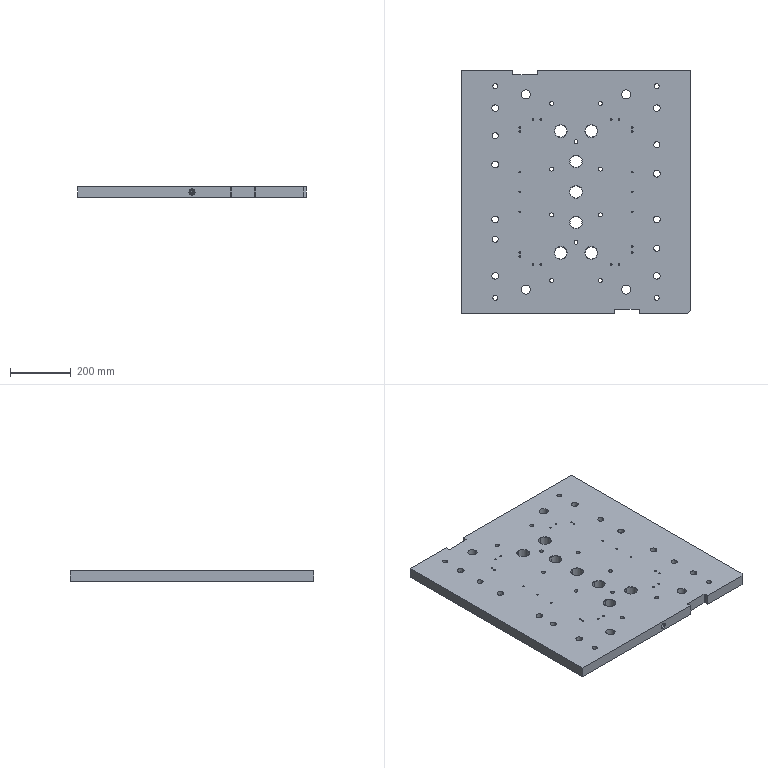Part | Creo | 1 solid | 678 faces | box 750 x 800 x 35 mm | volume 19950074 mm3 | cylinder 410 | plane 166 | cone 102 | commonest cylinder face diameters 4.199 x66 4.2 x66 8 x56 5.5 x44 9 x44 13 x20